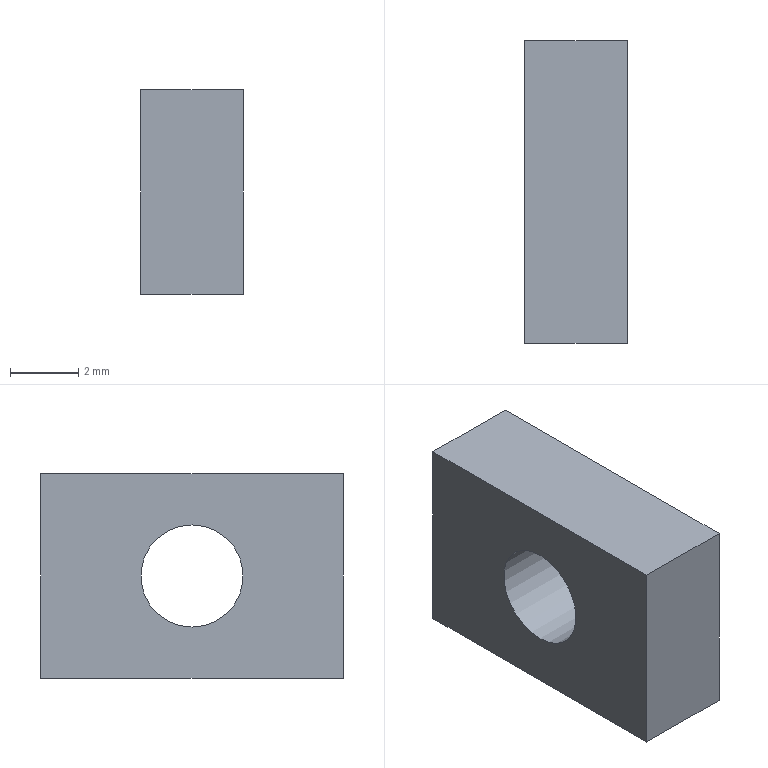Part | STEP file | solid 192 | 1 solid | 7 faces | box 3 x 8.885 x 6 mm | volume 138.722 mm3 | plane 6 | cylinder 1 | commonest cylinder face diameters 3 x1